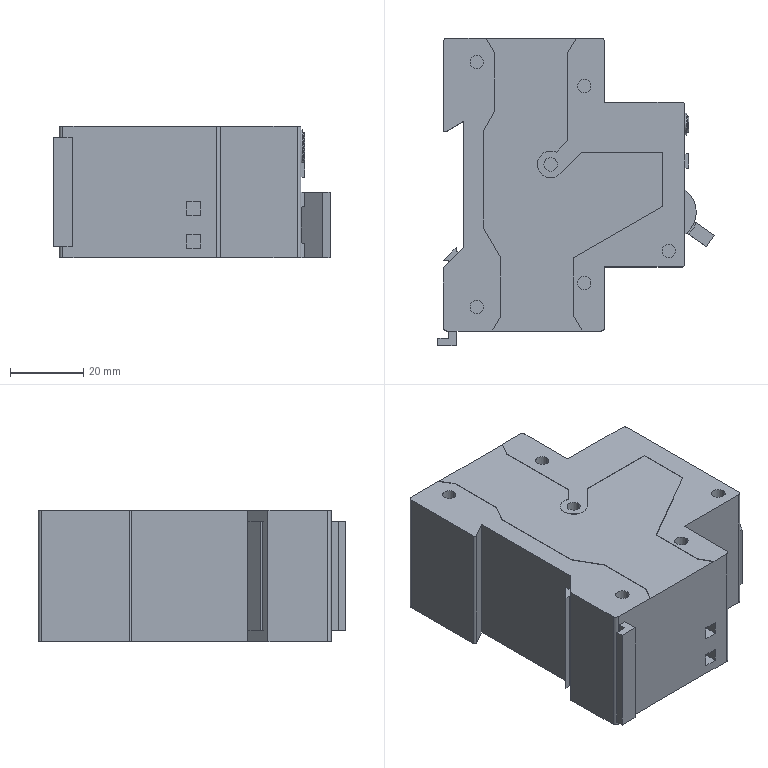Part | STEP file | circuit breaker DZ267LE-32-10 | 5 solids | 266 faces | box 75.5 x 84 x 36 mm | volume 154947 mm3 | plane 192 | cylinder 66 | spline 8 | commonest cylinder face diameters 3.667 x32 4.1 x8 4.5 x8 2 x6 7.333 x3 14 x3